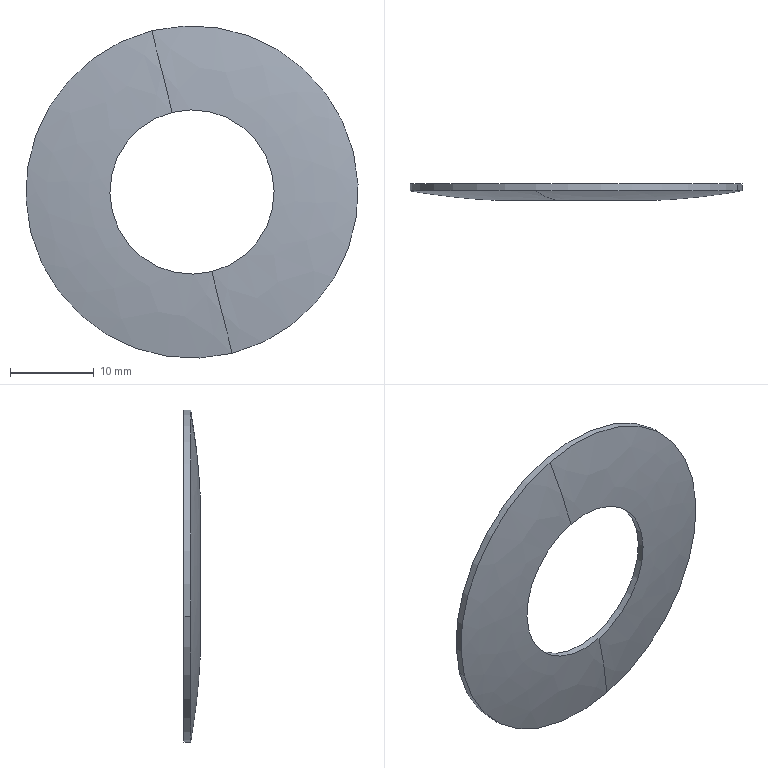Part | NX | features BREP 1 | 1 solid | 8 faces | box 39.654 x 1.932 x 39.654 mm | volume 696.294 mm3 | spline 4 | cylinder 4 | commonest cylinder face diameters 19.6 x2 39.654 x2
STEP:
#1=CARTESIAN_POINT('',(31.684,-43.121,19.794));
#2=VERTEX_POINT('',#1);
#3=CARTESIAN_POINT('',(17.229,-43.121,-4.232));
#4=VERTEX_POINT('',#3);
#5=CARTESIAN_POINT('',(36.47,-43.121,0.5537));
#6=DIRECTION('',(0.,-1.,0.));
#7=DIRECTION('',(-0.9704,0.,-0.2414));
#8=AXIS2_PLACEMENT_3D('',#5,#6,#7);
#9=CIRCLE('',#8,19.827);
#10=EDGE_CURVE('',#2,#4,#9,.T.);
#11=ORIENTED_EDGE('',*,*,#10,.F.);
#12=CARTESIAN_POINT('',(34.104,-44.236,10.064));
#13=VERTEX_POINT('',#12);
#14=CARTESIAN_POINT('',(31.684,-43.121,19.794));
#15=CARTESIAN_POINT('',(32.872,-44.213,15.02));
#16=CARTESIAN_POINT('',(34.104,-44.236,10.064));
#17=B_SPLINE_CURVE_WITH_KNOTS('',2,(#14,#15,#16),.UNSPECIFIED.,.F.,.F.,(3,3),(0.,1.),.PIECEWISE_BEZIER_KNOTS.);
#18=EDGE_CURVE('',#2,#13,#17,.T.);
#19=ORIENTED_EDGE('',*,*,#18,.T.);
#20=CARTESIAN_POINT('',(26.959,-44.236,-1.812));
#21=VERTEX_POINT('',#20);
#22=CARTESIAN_POINT('',(36.47,-44.236,0.5537));
#23=DIRECTION('',(0.,-1.,0.));
#24=DIRECTION('',(-0.9704,0.,-0.2414));
#25=AXIS2_PLACEMENT_3D('',#22,#23,#24);
#26=CIRCLE('',#25,9.8);
#27=EDGE_CURVE('',#13,#21,#26,.T.);
#28=ORIENTED_EDGE('',*,*,#27,.T.);
#29=CARTESIAN_POINT('',(38.835,-44.236,-8.957));
#30=VERTEX_POINT('',#29);
#31=CARTESIAN_POINT('',(36.47,-44.236,0.5537));
#32=DIRECTION('',(0.,-1.,0.));
#33=DIRECTION('',(-0.9704,0.,-0.2414));
#34=AXIS2_PLACEMENT_3D('',#31,#32,#33);
#35=CIRCLE('',#34,9.8);
#36=EDGE_CURVE('',#21,#30,#35,.T.);
#37=ORIENTED_EDGE('',*,*,#36,.T.);
#38=CARTESIAN_POINT('',(41.255,-43.121,-18.687));
#39=VERTEX_POINT('',#38);
#40=CARTESIAN_POINT('',(41.255,-43.121,-18.687));
#41=CARTESIAN_POINT('',(40.068,-44.213,-13.912));
#42=CARTESIAN_POINT('',(38.835,-44.236,-8.957));
#43=B_SPLINE_CURVE_WITH_KNOTS('',2,(#40,#41,#42),.UNSPECIFIED.,.F.,.F.,(3,3),(0.,1.),.PIECEWISE_BEZIER_KNOTS.);
#44=EDGE_CURVE('',#39,#30,#43,.T.);
#45=ORIENTED_EDGE('',*,*,#44,.F.);
#46=CARTESIAN_POINT('',(36.47,-43.121,0.5537));
#47=DIRECTION('',(0.,-1.,0.));
#48=DIRECTION('',(-0.9704,0.,-0.2414));
#49=AXIS2_PLACEMENT_3D('',#46,#47,#48);
#50=CIRCLE('',#49,19.827);
#51=EDGE_CURVE('',#4,#39,#50,.T.);
#52=ORIENTED_EDGE('',*,*,#51,.F.);
#53=EDGE_LOOP('',(#11,#19,#28,#37,#45,#52));
#54=FACE_BOUND('',#53,.T.);
#55=CARTESIAN_POINT('',(31.684,-43.121,19.794));
#56=CARTESIAN_POINT('',(-6.797,-43.121,10.223));
#57=CARTESIAN_POINT('',(2.774,-43.121,-28.258));
#58=CARTESIAN_POINT('',(41.255,-43.121,-18.687));
#59=CARTESIAN_POINT('',(32.872,-44.213,15.02));
#60=CARTESIAN_POINT('',(3.939,-44.213,7.824));
#61=CARTESIAN_POINT('',(11.135,-44.213,-21.108));
#62=CARTESIAN_POINT('',(40.068,-44.213,-13.912));
#63=CARTESIAN_POINT('',(34.104,-44.236,10.064));
#64=CARTESIAN_POINT('',(15.084,-44.236,5.333));
#65=CARTESIAN_POINT('',(19.814,-44.236,-13.687));
#66=CARTESIAN_POINT('',(38.835,-44.236,-8.957));
#67=(BOUNDED_SURFACE()B_SPLINE_SURFACE(2,3,((#55,#56,#57,#58),(#59,#60,#61,#62),(#63,#64,#65,#66)),.SURF_OF_REVOLUTION.,.F.,.F.,.F.)B_SPLINE_SURFACE_WITH_KNOTS((3,3),(4,4),(0.,1.),(0.,1.),.PIECEWISE_BEZIER_KNOTS.)GEOMETRIC_REPRESENTATION_ITEM()RATIONAL_B_SPLINE_SURFACE(((1.,0.3333,0.3333,1.),(1.,0.3333,0.3333,1.),(1.,0.3333,0.3333,1.)))REPRESENTATION_ITEM('')SURFACE());
#68=ADVANCED_FACE('',(#54),#67,.T.);
#69=CARTESIAN_POINT('',(34.104,-45.053,10.064));
#70=VERTEX_POINT('',#69);
#71=CARTESIAN_POINT('',(26.959,-45.053,-1.812));
#72=VERTEX_POINT('',#71);
#73=CARTESIAN_POINT('',(36.47,-45.053,0.5537));
#74=DIRECTION('',(0.,-1.,0.));
#75=DIRECTION('',(-0.9704,0.,-0.2414));
#76=AXIS2_PLACEMENT_3D('',#73,#74,#75);
#77=CIRCLE('',#76,9.8);
#78=EDGE_CURVE('',#70,#72,#77,.T.);
#79=ORIENTED_EDGE('',*,*,#78,.F.);
#80=CARTESIAN_POINT('',(31.684,-43.937,19.794));
#81=VERTEX_POINT('',#80);
#82=CARTESIAN_POINT('',(34.104,-45.053,10.064));
#83=CARTESIAN_POINT('',(32.888,-44.826,14.954));
#84=CARTESIAN_POINT('',(31.684,-43.937,19.794));
#85=B_SPLINE_CURVE_WITH_KNOTS('',2,(#82,#83,#84),.UNSPECIFIED.,.F.,.F.,(3,3),(0.,1.),.PIECEWISE_BEZIER_KNOTS.);
#86=EDGE_CURVE('',#70,#81,#85,.T.);
#87=ORIENTED_EDGE('',*,*,#86,.T.);
#88=CARTESIAN_POINT('',(17.229,-43.937,-4.232));
#89=VERTEX_POINT('',#88);
#90=CARTESIAN_POINT('',(36.47,-43.937,0.5537));
#91=DIRECTION('',(0.,-1.,0.));
#92=DIRECTION('',(-0.9704,0.,-0.2414));
#93=AXIS2_PLACEMENT_3D('',#90,#91,#92);
#94=CIRCLE('',#93,19.827);
#95=EDGE_CURVE('',#81,#89,#94,.T.);
#96=ORIENTED_EDGE('',*,*,#95,.T.);
#97=CARTESIAN_POINT('',(41.255,-43.937,-18.687));
#98=VERTEX_POINT('',#97);
#99=CARTESIAN_POINT('',(36.47,-43.937,0.5537));
#100=DIRECTION('',(0.,-1.,0.));
#101=DIRECTION('',(-0.9704,0.,-0.2414));
#102=AXIS2_PLACEMENT_3D('',#99,#100,#101);
#103=CIRCLE('',#102,19.827);
#104=EDGE_CURVE('',#89,#98,#103,.T.);
#105=ORIENTED_EDGE('',*,*,#104,.T.);
#106=CARTESIAN_POINT('',(38.835,-45.053,-8.957));
#107=VERTEX_POINT('',#106);
#108=CARTESIAN_POINT('',(38.835,-45.053,-8.957));
#109=CARTESIAN_POINT('',(40.051,-44.826,-13.846));
#110=CARTESIAN_POINT('',(41.255,-43.937,-18.687));
#111=B_SPLINE_CURVE_WITH_KNOTS('',2,(#108,#109,#110),.UNSPECIFIED.,.F.,.F.,(3,3),(0.,1.),.PIECEWISE_BEZIER_KNOTS.);
#112=EDGE_CURVE('',#107,#98,#111,.T.);
#113=ORIENTED_EDGE('',*,*,#112,.F.);
#114=CARTESIAN_POINT('',(36.47,-45.053,0.5537));
#115=DIRECTION('',(0.,-1.,0.));
#116=DIRECTION('',(-0.9704,0.,-0.2414));
#117=AXIS2_PLACEMENT_3D('',#114,#115,#116);
#118=CIRCLE('',#117,9.8);
#119=EDGE_CURVE('',#72,#107,#118,.T.);
#120=ORIENTED_EDGE('',*,*,#119,.F.);
#121=EDGE_LOOP('',(#79,#87,#96,#105,#113,#120));
#122=FACE_BOUND('',#121,.T.);
#123=CARTESIAN_POINT('',(34.104,-45.053,10.064));
#124=CARTESIAN_POINT('',(15.084,-45.053,5.333));
#125=CARTESIAN_POINT('',(19.814,-45.053,-13.687));
#126=CARTESIAN_POINT('',(38.835,-45.053,-8.957));
#127=CARTESIAN_POINT('',(32.888,-44.826,14.954));
#128=CARTESIAN_POINT('',(4.088,-44.826,7.791));
#129=CARTESIAN_POINT('',(11.251,-44.826,-21.009));
#130=CARTESIAN_POINT('',(40.051,-44.826,-13.846));
#131=CARTESIAN_POINT('',(31.684,-43.937,19.794));
#132=CARTESIAN_POINT('',(-6.797,-43.937,10.223));
#133=CARTESIAN_POINT('',(2.774,-43.937,-28.258));
#134=CARTESIAN_POINT('',(41.255,-43.937,-18.687));
#135=(BOUNDED_SURFACE()B_SPLINE_SURFACE(2,3,((#123,#124,#125,#126),(#127,#128,#129,#130),(#131,#132,#133,#134)),.SURF_OF_REVOLUTION.,.F.,.F.,.F.)B_SPLINE_SURFACE_WITH_KNOTS((3,3),(4,4),(0.,1.),(0.,1.),.PIECEWISE_BEZIER_KNOTS.)GEOMETRIC_REPRESENTATION_ITEM()RATIONAL_B_SPLINE_SURFACE(((1.,0.3333,0.3333,1.),(1.,0.3333,0.3333,1.),(1.,0.3333,0.3333,1.)))REPRESENTATION_ITEM('')SURFACE());
#136=ADVANCED_FACE('',(#122),#135,.T.);
#137=CARTESIAN_POINT('',(45.98,-44.236,2.919));
#138=VERTEX_POINT('',#137);
#139=CARTESIAN_POINT('',(36.47,-44.236,0.5537));
#140=DIRECTION('',(0.,-1.,0.));
#141=DIRECTION('',(-0.9704,0.,-0.2414));
#142=AXIS2_PLACEMENT_3D('',#139,#140,#141);
#143=CIRCLE('',#142,9.8);
#144=EDGE_CURVE('',#138,#13,#143,.T.);
#145=ORIENTED_EDGE('',*,*,#144,.F.);
#146=CARTESIAN_POINT('',(45.98,-45.053,2.919));
#147=VERTEX_POINT('',#146);
#148=CARTESIAN_POINT('',(45.98,-45.053,2.919));
#149=DIRECTION('',(0.,-1.,0.));
#150=VECTOR('',#149,1000.);
#151=LINE('',#148,#150);
#152=EDGE_CURVE('',#147,#138,#151,.F.);
#153=ORIENTED_EDGE('',*,*,#152,.F.);
#154=CARTESIAN_POINT('',(36.47,-45.053,0.5537));
#155=DIRECTION('',(0.,-1.,0.));
#156=DIRECTION('',(-0.9704,0.,-0.2414));
#157=AXIS2_PLACEMENT_3D('',#154,#155,#156);
#158=CIRCLE('',#157,9.8);
#159=EDGE_CURVE('',#147,#70,#158,.T.);
#160=ORIENTED_EDGE('',*,*,#159,.T.);
#161=ORIENTED_EDGE('',*,*,#78,.T.);
#162=CARTESIAN_POINT('',(26.959,-45.053,-1.812));
#163=DIRECTION('',(0.,-1.,0.));
#164=VECTOR('',#163,1000.);
#165=LINE('',#162,#164);
#166=EDGE_CURVE('',#72,#21,#165,.F.);
#167=ORIENTED_EDGE('',*,*,#166,.T.);
#168=ORIENTED_EDGE('',*,*,#27,.F.);
#169=EDGE_LOOP('',(#145,#153,#160,#161,#167,#168));
#170=FACE_BOUND('',#169,.T.);
#171=CARTESIAN_POINT('',(36.47,-45.053,0.5537));
#172=DIRECTION('',(0.,-1.,0.));
#173=DIRECTION('',(0.9704,0.,0.2414));
#174=AXIS2_PLACEMENT_3D('',#171,#172,#173);
#175=CYLINDRICAL_SURFACE('',#174,9.8);
#176=ADVANCED_FACE('',(#170),#175,.F.);
#177=ORIENTED_EDGE('',*,*,#51,.T.);
#178=CARTESIAN_POINT('',(55.71,-43.121,5.339));
#179=VERTEX_POINT('',#178);
#180=CARTESIAN_POINT('',(36.47,-43.121,0.5537));
#181=DIRECTION('',(0.,-1.,0.));
#182=DIRECTION('',(-0.9704,0.,-0.2414));
#183=AXIS2_PLACEMENT_3D('',#180,#181,#182);
#184=CIRCLE('',#183,19.827);
#185=EDGE_CURVE('',#39,#179,#184,.T.);
#186=ORIENTED_EDGE('',*,*,#185,.T.);
#187=CARTESIAN_POINT('',(55.71,-43.937,5.339));
#188=VERTEX_POINT('',#187);
#189=CARTESIAN_POINT('',(55.71,-45.053,5.339));
#190=DIRECTION('',(0.,-1.,0.));
#191=VECTOR('',#190,1000.);
#192=LINE('',#189,#191);
#193=EDGE_CURVE('',#188,#179,#192,.F.);
#194=ORIENTED_EDGE('',*,*,#193,.F.);
#195=CARTESIAN_POINT('',(36.47,-43.937,0.5537));
#196=DIRECTION('',(0.,-1.,0.));
#197=DIRECTION('',(-0.9704,0.,-0.2414));
#198=AXIS2_PLACEMENT_3D('',#195,#196,#197);
#199=CIRCLE('',#198,19.827);
#200=EDGE_CURVE('',#98,#188,#199,.T.);
#201=ORIENTED_EDGE('',*,*,#200,.F.);
#202=ORIENTED_EDGE('',*,*,#104,.F.);
#203=CARTESIAN_POINT('',(17.229,-45.053,-4.232));
#204=DIRECTION('',(0.,-1.,0.));
#205=VECTOR('',#204,1000.);
#206=LINE('',#203,#205);
#207=EDGE_CURVE('',#89,#4,#206,.F.);
#208=ORIENTED_EDGE('',*,*,#207,.T.);
#209=EDGE_LOOP('',(#177,#186,#194,#201,#202,#208));
#210=FACE_BOUND('',#209,.T.);
#211=CARTESIAN_POINT('',(36.47,-45.053,0.5537));
#212=DIRECTION('',(0.,-1.,0.));
#213=DIRECTION('',(0.9704,0.,0.2414));
#214=AXIS2_PLACEMENT_3D('',#211,#212,#213);
#215=CYLINDRICAL_SURFACE('',#214,19.827);
#216=ADVANCED_FACE('',(#210),#215,.T.);
#217=ORIENTED_EDGE('',*,*,#86,.F.);
#218=ORIENTED_EDGE('',*,*,#159,.F.);
#219=CARTESIAN_POINT('',(36.47,-45.053,0.5537));
#220=DIRECTION('',(0.,-1.,0.));
#221=DIRECTION('',(-0.9704,0.,-0.2414));
#222=AXIS2_PLACEMENT_3D('',#219,#220,#221);
#223=CIRCLE('',#222,9.8);
#224=EDGE_CURVE('',#107,#147,#223,.T.);
#225=ORIENTED_EDGE('',*,*,#224,.F.);
#226=ORIENTED_EDGE('',*,*,#112,.T.);
#227=ORIENTED_EDGE('',*,*,#200,.T.);
#228=CARTESIAN_POINT('',(36.47,-43.937,0.5537));
#229=DIRECTION('',(0.,-1.,0.));
#230=DIRECTION('',(-0.9704,0.,-0.2414));
#231=AXIS2_PLACEMENT_3D('',#228,#229,#230);
#232=CIRCLE('',#231,19.827);
#233=EDGE_CURVE('',#188,#81,#232,.T.);
#234=ORIENTED_EDGE('',*,*,#233,.T.);
#235=EDGE_LOOP('',(#217,#218,#225,#226,#227,#234));
#236=FACE_BOUND('',#235,.T.);
#237=CARTESIAN_POINT('',(38.835,-45.053,-8.957));
#238=CARTESIAN_POINT('',(57.855,-45.053,-4.226));
#239=CARTESIAN_POINT('',(53.125,-45.053,14.795));
#240=CARTESIAN_POINT('',(34.104,-45.053,10.064));
#241=CARTESIAN_POINT('',(40.051,-44.826,-13.846));
#242=CARTESIAN_POINT('',(68.851,-44.826,-6.683));
#243=CARTESIAN_POINT('',(61.688,-44.826,22.117));
#244=CARTESIAN_POINT('',(32.888,-44.826,14.954));
#245=CARTESIAN_POINT('',(41.255,-43.937,-18.687));
#246=CARTESIAN_POINT('',(79.736,-43.937,-9.116));
#247=CARTESIAN_POINT('',(70.165,-43.937,29.365));
#248=CARTESIAN_POINT('',(31.684,-43.937,19.794));
#249=(BOUNDED_SURFACE()B_SPLINE_SURFACE(2,3,((#237,#238,#239,#240),(#241,#242,#243,#244),(#245,#246,#247,#248)),.SURF_OF_REVOLUTION.,.F.,.F.,.F.)B_SPLINE_SURFACE_WITH_KNOTS((3,3),(4,4),(0.,1.),(0.,1.),.PIECEWISE_BEZIER_KNOTS.)GEOMETRIC_REPRESENTATION_ITEM()RATIONAL_B_SPLINE_SURFACE(((1.,0.3333,0.3333,1.),(1.,0.3333,0.3333,1.),(1.,0.3333,0.3333,1.)))REPRESENTATION_ITEM('')SURFACE());
#250=ADVANCED_FACE('',(#236),#249,.T.);
#251=ORIENTED_EDGE('',*,*,#193,.T.);
#252=CARTESIAN_POINT('',(36.47,-43.121,0.5537));
#253=DIRECTION('',(0.,-1.,0.));
#254=DIRECTION('',(-0.9704,0.,-0.2414));
#255=AXIS2_PLACEMENT_3D('',#252,#253,#254);
#256=CIRCLE('',#255,19.827);
#257=EDGE_CURVE('',#179,#2,#256,.T.);
#258=ORIENTED_EDGE('',*,*,#257,.T.);
#259=ORIENTED_EDGE('',*,*,#10,.T.);
#260=ORIENTED_EDGE('',*,*,#207,.F.);
#261=ORIENTED_EDGE('',*,*,#95,.F.);
#262=ORIENTED_EDGE('',*,*,#233,.F.);
#263=EDGE_LOOP('',(#251,#258,#259,#260,#261,#262));
#264=FACE_BOUND('',#263,.T.);
#265=CARTESIAN_POINT('',(36.47,-45.053,0.5537));
#266=DIRECTION('',(0.,-1.,0.));
#267=DIRECTION('',(0.9704,0.,0.2414));
#268=AXIS2_PLACEMENT_3D('',#265,#266,#267);
#269=CYLINDRICAL_SURFACE('',#268,19.827);
#270=ADVANCED_FACE('',(#264),#269,.T.);
#271=ORIENTED_EDGE('',*,*,#18,.F.);
#272=ORIENTED_EDGE('',*,*,#257,.F.);
#273=ORIENTED_EDGE('',*,*,#185,.F.);
#274=ORIENTED_EDGE('',*,*,#44,.T.);
#275=CARTESIAN_POINT('',(36.47,-44.236,0.5537));
#276=DIRECTION('',(0.,-1.,0.));
#277=DIRECTION('',(-0.9704,0.,-0.2414));
#278=AXIS2_PLACEMENT_3D('',#275,#276,#277);
#279=CIRCLE('',#278,9.8);
#280=EDGE_CURVE('',#30,#138,#279,.T.);
#281=ORIENTED_EDGE('',*,*,#280,.T.);
#282=ORIENTED_EDGE('',*,*,#144,.T.);
#283=EDGE_LOOP('',(#271,#272,#273,#274,#281,#282));
#284=FACE_BOUND('',#283,.T.);
#285=CARTESIAN_POINT('',(41.255,-43.121,-18.687));
#286=CARTESIAN_POINT('',(79.736,-43.121,-9.116));
#287=CARTESIAN_POINT('',(70.165,-43.121,29.365));
#288=CARTESIAN_POINT('',(31.684,-43.121,19.794));
#289=CARTESIAN_POINT('',(40.068,-44.213,-13.912));
#290=CARTESIAN_POINT('',(69.,-44.213,-6.717));
#291=CARTESIAN_POINT('',(61.804,-44.213,22.216));
#292=CARTESIAN_POINT('',(32.872,-44.213,15.02));
#293=CARTESIAN_POINT('',(38.835,-44.236,-8.957));
#294=CARTESIAN_POINT('',(57.855,-44.236,-4.226));
#295=CARTESIAN_POINT('',(53.125,-44.236,14.795));
#296=CARTESIAN_POINT('',(34.104,-44.236,10.064));
#297=(BOUNDED_SURFACE()B_SPLINE_SURFACE(2,3,((#285,#286,#287,#288),(#289,#290,#291,#292),(#293,#294,#295,#296)),.SURF_OF_REVOLUTION.,.F.,.F.,.F.)B_SPLINE_SURFACE_WITH_KNOTS((3,3),(4,4),(0.,1.),(0.,1.),.PIECEWISE_BEZIER_KNOTS.)GEOMETRIC_REPRESENTATION_ITEM()RATIONAL_B_SPLINE_SURFACE(((1.,0.3333,0.3333,1.),(1.,0.3333,0.3333,1.),(1.,0.3333,0.3333,1.)))REPRESENTATION_ITEM('')SURFACE());
#298=ADVANCED_FACE('',(#284),#297,.T.);
#299=ORIENTED_EDGE('',*,*,#152,.T.);
#300=ORIENTED_EDGE('',*,*,#280,.F.);
#301=ORIENTED_EDGE('',*,*,#36,.F.);
#302=ORIENTED_EDGE('',*,*,#166,.F.);
#303=ORIENTED_EDGE('',*,*,#119,.T.);
#304=ORIENTED_EDGE('',*,*,#224,.T.);
#305=EDGE_LOOP('',(#299,#300,#301,#302,#303,#304));
#306=FACE_BOUND('',#305,.T.);
#307=CARTESIAN_POINT('',(36.47,-45.053,0.5537));
#308=DIRECTION('',(0.,-1.,0.));
#309=DIRECTION('',(0.9704,0.,0.2414));
#310=AXIS2_PLACEMENT_3D('',#307,#308,#309);
#311=CYLINDRICAL_SURFACE('',#310,9.8);
#312=ADVANCED_FACE('',(#306),#311,.F.);
#313=CLOSED_SHELL('',(#68,#136,#176,#216,#250,#270,#298,#312));
#314=MANIFOLD_SOLID_BREP('',#313);
#315=(LENGTH_UNIT()NAMED_UNIT(*)SI_UNIT(.MILLI.,.METRE.));
#316=UNCERTAINTY_MEASURE_WITH_UNIT(LENGTH_MEASURE(0.00001),#315,'','');
#317=(NAMED_UNIT(*)PLANE_ANGLE_UNIT()SI_UNIT($,.RADIAN.));
#318=(NAMED_UNIT(*)SI_UNIT($,.STERADIAN.)SOLID_ANGLE_UNIT());
#319=(GEOMETRIC_REPRESENTATION_CONTEXT(3)GLOBAL_UNCERTAINTY_ASSIGNED_CONTEXT((#316))GLOBAL_UNIT_ASSIGNED_CONTEXT((#315,#317,#318))REPRESENTATION_CONTEXT('',''));
#320=ADVANCED_BREP_SHAPE_REPRESENTATION('',(#314),#319);